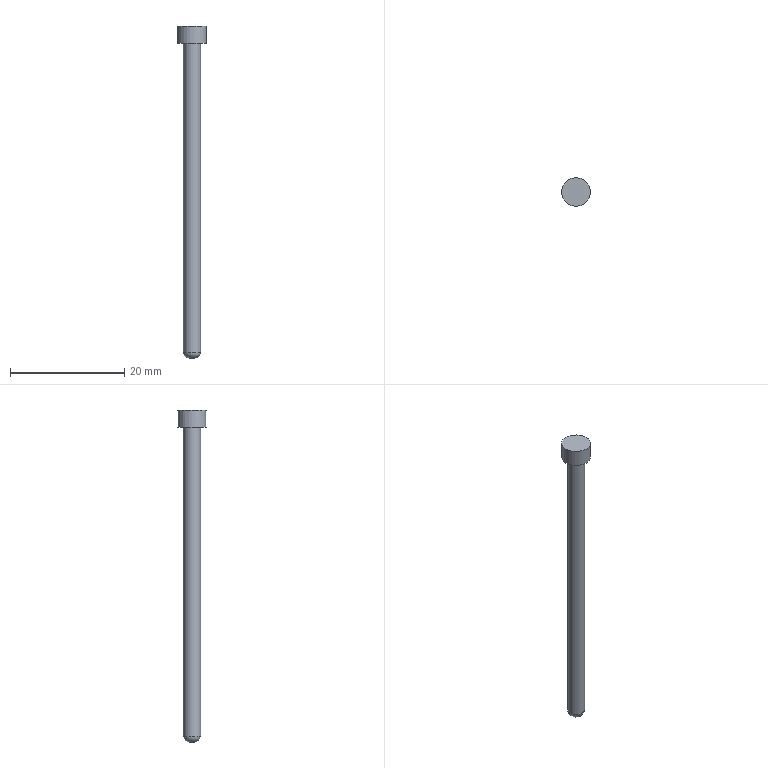Part | NX | features PG_666 2 | 1 solid | 6 faces | box 5 x 5 x 58 mm | volume 446.214 mm3 | plane 3 | cylinder 2 | torus 1 | commonest cylinder face diameters 3.001 x1 5 x1
STEP:
#1=CARTESIAN_POINT('',(2690.539,-918.401,851.716));
#2=VERTEX_POINT('',#1);
#3=CARTESIAN_POINT('',(2692.04,-918.401,851.716));
#4=DIRECTION('',(0.,0.,1.));
#5=DIRECTION('',(-1.,0.,0.));
#6=AXIS2_PLACEMENT_3D('',#3,#4,#5);
#7=CIRCLE('',#6,1.5);
#8=EDGE_CURVE('',#2,#2,#7,.F.);
#9=ORIENTED_EDGE('',*,*,#8,.F.);
#10=EDGE_LOOP('',(#9));
#11=FACE_BOUND('',#10,.T.);
#12=CARTESIAN_POINT('',(2690.539,-918.401,905.716));
#13=VERTEX_POINT('',#12);
#14=CARTESIAN_POINT('',(2692.04,-918.401,905.716));
#15=DIRECTION('',(0.,0.,1.));
#16=DIRECTION('',(-1.,0.,0.));
#17=AXIS2_PLACEMENT_3D('',#14,#15,#16);
#18=CIRCLE('',#17,1.5);
#19=EDGE_CURVE('',#13,#13,#18,.F.);
#20=ORIENTED_EDGE('',*,*,#19,.T.);
#21=EDGE_LOOP('',(#20));
#22=FACE_BOUND('',#21,.T.);
#23=CARTESIAN_POINT('',(2692.04,-918.401,855.716));
#24=DIRECTION('',(0.,0.,1.));
#25=DIRECTION('',(1.,0.,0.));
#26=AXIS2_PLACEMENT_3D('',#23,#24,#25);
#27=CYLINDRICAL_SURFACE('',#26,1.5);
#28=ADVANCED_FACE('',(#11,#22),#27,.T.);
#29=CARTESIAN_POINT('',(2691.539,-918.401,850.716));
#30=VERTEX_POINT('',#29);
#31=CARTESIAN_POINT('',(2692.04,-918.401,850.716));
#32=DIRECTION('',(0.,0.,1.));
#33=DIRECTION('',(-1.,0.,0.));
#34=AXIS2_PLACEMENT_3D('',#31,#32,#33);
#35=CIRCLE('',#34,0.5005);
#36=EDGE_CURVE('',#30,#30,#35,.T.);
#37=ORIENTED_EDGE('',*,*,#36,.F.);
#38=EDGE_LOOP('',(#37));
#39=FACE_BOUND('',#38,.T.);
#40=CARTESIAN_POINT('',(2692.04,-918.401,850.716));
#41=DIRECTION('',(0.,0.,-1.));
#42=DIRECTION('',(-1.,0.,0.));
#43=AXIS2_PLACEMENT_3D('',#40,#41,#42);
#44=PLANE('',#43);
#45=ADVANCED_FACE('',(#39),#44,.T.);
#46=CARTESIAN_POINT('',(2694.54,-918.401,908.716));
#47=VERTEX_POINT('',#46);
#48=CARTESIAN_POINT('',(2692.04,-918.401,908.716));
#49=DIRECTION('',(0.,0.,1.));
#50=DIRECTION('',(1.,0.,0.));
#51=AXIS2_PLACEMENT_3D('',#48,#49,#50);
#52=CIRCLE('',#51,2.5);
#53=EDGE_CURVE('',#47,#47,#52,.T.);
#54=ORIENTED_EDGE('',*,*,#53,.T.);
#55=EDGE_LOOP('',(#54));
#56=FACE_BOUND('',#55,.T.);
#57=CARTESIAN_POINT('',(2692.04,-918.401,908.716));
#58=DIRECTION('',(0.,0.,1.));
#59=DIRECTION('',(1.,0.,0.));
#60=AXIS2_PLACEMENT_3D('',#57,#58,#59);
#61=PLANE('',#60);
#62=ADVANCED_FACE('',(#56),#61,.T.);
#63=ORIENTED_EDGE('',*,*,#19,.F.);
#64=EDGE_LOOP('',(#63));
#65=FACE_BOUND('',#64,.T.);
#66=CARTESIAN_POINT('',(2694.54,-918.401,905.716));
#67=VERTEX_POINT('',#66);
#68=CARTESIAN_POINT('',(2692.04,-918.401,905.716));
#69=DIRECTION('',(0.,0.,-1.));
#70=DIRECTION('',(1.,0.,0.));
#71=AXIS2_PLACEMENT_3D('',#68,#69,#70);
#72=CIRCLE('',#71,2.5);
#73=EDGE_CURVE('',#67,#67,#72,.T.);
#74=ORIENTED_EDGE('',*,*,#73,.T.);
#75=EDGE_LOOP('',(#74));
#76=FACE_BOUND('',#75,.T.);
#77=CARTESIAN_POINT('',(2692.04,-918.401,905.716));
#78=DIRECTION('',(0.,0.,-1.));
#79=DIRECTION('',(-1.,0.,0.));
#80=AXIS2_PLACEMENT_3D('',#77,#78,#79);
#81=PLANE('',#80);
#82=ADVANCED_FACE('',(#65,#76),#81,.T.);
#83=ORIENTED_EDGE('',*,*,#53,.F.);
#84=EDGE_LOOP('',(#83));
#85=FACE_BOUND('',#84,.T.);
#86=ORIENTED_EDGE('',*,*,#73,.F.);
#87=EDGE_LOOP('',(#86));
#88=FACE_BOUND('',#87,.T.);
#89=CARTESIAN_POINT('',(2692.04,-918.401,905.716));
#90=DIRECTION('',(0.,0.,1.));
#91=DIRECTION('',(1.,0.,0.));
#92=AXIS2_PLACEMENT_3D('',#89,#90,#91);
#93=CYLINDRICAL_SURFACE('',#92,2.5);
#94=ADVANCED_FACE('',(#85,#88),#93,.T.);
#95=ORIENTED_EDGE('',*,*,#36,.T.);
#96=EDGE_LOOP('',(#95));
#97=FACE_BOUND('',#96,.T.);
#98=ORIENTED_EDGE('',*,*,#8,.T.);
#99=EDGE_LOOP('',(#98));
#100=FACE_BOUND('',#99,.T.);
#101=CARTESIAN_POINT('',(2692.04,-918.401,851.716));
#102=DIRECTION('',(0.,0.,-1.));
#103=DIRECTION('',(-1.,0.,0.));
#104=AXIS2_PLACEMENT_3D('',#101,#102,#103);
#105=DEGENERATE_TOROIDAL_SURFACE('',#104,0.5005,1.,.T.);
#106=ADVANCED_FACE('',(#97,#100),#105,.T.);
#107=CLOSED_SHELL('',(#28,#45,#62,#82,#94,#106));
#108=MANIFOLD_SOLID_BREP('',#107);
#109=(LENGTH_UNIT()NAMED_UNIT(*)SI_UNIT(.MILLI.,.METRE.));
#110=UNCERTAINTY_MEASURE_WITH_UNIT(LENGTH_MEASURE(0.00001),#109,'','');
#111=(NAMED_UNIT(*)PLANE_ANGLE_UNIT()SI_UNIT($,.RADIAN.));
#112=(NAMED_UNIT(*)SI_UNIT($,.STERADIAN.)SOLID_ANGLE_UNIT());
#113=(GEOMETRIC_REPRESENTATION_CONTEXT(3)GLOBAL_UNCERTAINTY_ASSIGNED_CONTEXT((#110))GLOBAL_UNIT_ASSIGNED_CONTEXT((#109,#111,#112))REPRESENTATION_CONTEXT('',''));
#114=ADVANCED_BREP_SHAPE_REPRESENTATION('',(#108),#113);